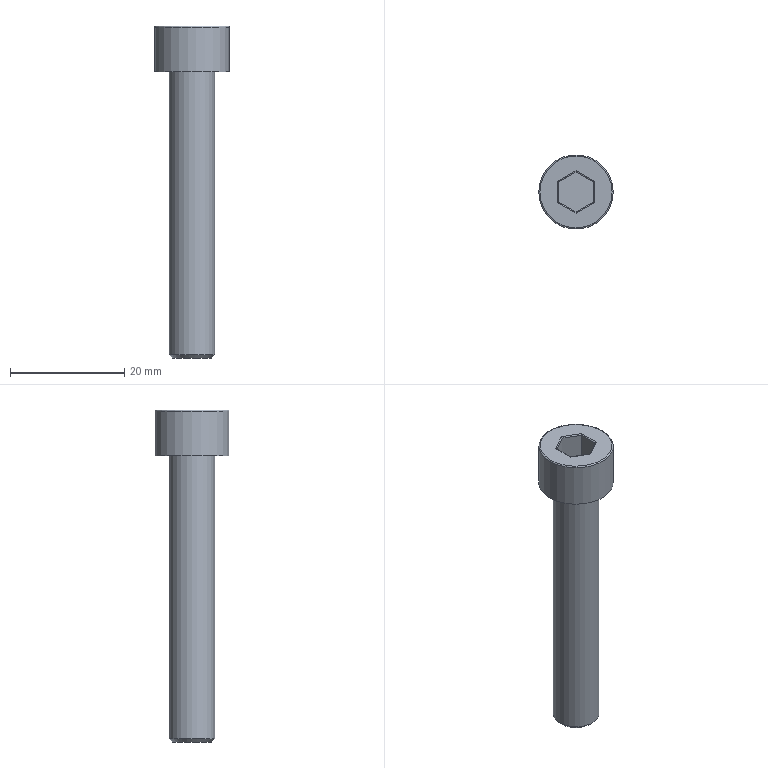Part | STEP file | 200 mesh_id666_x | 1 solid | 20 faces | box 13 x 13 x 58 mm | volume 3414 mm3 | plane 10 | cylinder 8 | torus 1 | cone 1 | commonest cylinder face diameters 0.4 x6 8 x1 13 x1
STEP:
#1=CARTESIAN_POINT('',(-16684.084,-4164.367,41.2));
#2=VERTEX_POINT('',#1);
#3=CARTESIAN_POINT('',(-16680.884,-4166.214,41.2));
#4=VERTEX_POINT('',#3);
#5=CARTESIAN_POINT('',(-16680.984,-4166.156,41.2));
#6=DIRECTION('',(0.866,-0.5,0.));
#7=VECTOR('',#6,1.);
#8=LINE('',#5,#7);
#9=EDGE_CURVE('',#2,#4,#8,.T.);
#10=ORIENTED_EDGE('',*,*,#9,.F.);
#11=CARTESIAN_POINT('',(-16684.084,-4160.672,41.2));
#12=VERTEX_POINT('',#11);
#13=CARTESIAN_POINT('',(-16684.084,-4164.251,41.2));
#14=DIRECTION('',(0.,-1.,0.));
#15=VECTOR('',#14,1.);
#16=LINE('',#13,#15);
#17=EDGE_CURVE('',#12,#2,#16,.T.);
#18=ORIENTED_EDGE('',*,*,#17,.F.);
#19=CARTESIAN_POINT('',(-16680.884,-4158.824,41.2));
#20=VERTEX_POINT('',#19);
#21=CARTESIAN_POINT('',(-16683.984,-4160.614,41.2));
#22=DIRECTION('',(-0.866,-0.5,0.));
#23=VECTOR('',#22,1.);
#24=LINE('',#21,#23);
#25=EDGE_CURVE('',#20,#12,#24,.T.);
#26=ORIENTED_EDGE('',*,*,#25,.F.);
#27=CARTESIAN_POINT('',(-16677.684,-4160.672,41.2));
#28=VERTEX_POINT('',#27);
#29=CARTESIAN_POINT('',(-16680.784,-4158.882,41.2));
#30=DIRECTION('',(-0.866,0.5,0.));
#31=VECTOR('',#30,1.);
#32=LINE('',#29,#31);
#33=EDGE_CURVE('',#28,#20,#32,.T.);
#34=ORIENTED_EDGE('',*,*,#33,.F.);
#35=CARTESIAN_POINT('',(-16677.684,-4164.367,41.2));
#36=VERTEX_POINT('',#35);
#37=CARTESIAN_POINT('',(-16677.684,-4160.787,41.2));
#38=DIRECTION('',(0.,1.,0.));
#39=VECTOR('',#38,1.);
#40=LINE('',#37,#39);
#41=EDGE_CURVE('',#36,#28,#40,.T.);
#42=ORIENTED_EDGE('',*,*,#41,.F.);
#43=CARTESIAN_POINT('',(-16677.784,-4164.424,41.2));
#44=DIRECTION('',(0.866,0.5,0.));
#45=VECTOR('',#44,1.);
#46=LINE('',#43,#45);
#47=EDGE_CURVE('',#4,#36,#46,.T.);
#48=ORIENTED_EDGE('',*,*,#47,.F.);
#49=EDGE_LOOP('',(#10,#18,#26,#34,#42,#48));
#50=FACE_BOUND('',#49,.T.);
#51=CARTESIAN_POINT('',(-16674.584,-4162.519,41.2));
#52=VERTEX_POINT('',#51);
#53=CARTESIAN_POINT('',(-16680.884,-4162.519,41.2));
#54=DIRECTION('',(0.,0.,-1.));
#55=DIRECTION('',(1.,0.,0.));
#56=AXIS2_PLACEMENT_3D('',#53,#54,#55);
#57=CIRCLE('',#56,6.3);
#58=EDGE_CURVE('',#52,#52,#57,.T.);
#59=ORIENTED_EDGE('',*,*,#58,.F.);
#60=EDGE_LOOP('',(#59));
#61=FACE_BOUND('',#60,.T.);
#62=CARTESIAN_POINT('',(-16680.884,-4162.519,41.2));
#63=DIRECTION('',(0.,0.,1.));
#64=DIRECTION('',(1.,0.,0.));
#65=AXIS2_PLACEMENT_3D('',#62,#63,#64);
#66=PLANE('',#65);
#67=ADVANCED_FACE('',(#50,#61),#66,.T.);
#68=CARTESIAN_POINT('',(-16684.884,-4162.519,-16.2));
#69=VERTEX_POINT('',#68);
#70=CARTESIAN_POINT('',(-16680.884,-4162.519,-16.2));
#71=DIRECTION('',(0.,0.,1.));
#72=DIRECTION('',(-1.,0.,0.));
#73=AXIS2_PLACEMENT_3D('',#70,#71,#72);
#74=CIRCLE('',#73,4.);
#75=EDGE_CURVE('',#69,#69,#74,.T.);
#76=ORIENTED_EDGE('',*,*,#75,.T.);
#77=EDGE_LOOP('',(#76));
#78=FACE_BOUND('',#77,.T.);
#79=CARTESIAN_POINT('',(-16684.884,-4162.519,33.2));
#80=VERTEX_POINT('',#79);
#81=CARTESIAN_POINT('',(-16680.884,-4162.519,33.2));
#82=DIRECTION('',(0.,0.,-1.));
#83=DIRECTION('',(-1.,0.,0.));
#84=AXIS2_PLACEMENT_3D('',#81,#82,#83);
#85=CIRCLE('',#84,4.);
#86=EDGE_CURVE('',#80,#80,#85,.T.);
#87=ORIENTED_EDGE('',*,*,#86,.T.);
#88=EDGE_LOOP('',(#87));
#89=FACE_BOUND('',#88,.T.);
#90=CARTESIAN_POINT('',(-16680.884,-4162.519,33.2));
#91=DIRECTION('',(0.,0.,-1.));
#92=DIRECTION('',(1.,0.,0.));
#93=AXIS2_PLACEMENT_3D('',#90,#91,#92);
#94=CYLINDRICAL_SURFACE('',#93,4.);
#95=ADVANCED_FACE('',(#78,#89),#94,.T.);
#96=ORIENTED_EDGE('',*,*,#86,.F.);
#97=EDGE_LOOP('',(#96));
#98=FACE_BOUND('',#97,.T.);
#99=CARTESIAN_POINT('',(-16687.384,-4162.519,33.2));
#100=VERTEX_POINT('',#99);
#101=CARTESIAN_POINT('',(-16680.884,-4162.519,33.2));
#102=DIRECTION('',(0.,0.,-1.));
#103=DIRECTION('',(-1.,0.,0.));
#104=AXIS2_PLACEMENT_3D('',#101,#102,#103);
#105=CIRCLE('',#104,6.5);
#106=EDGE_CURVE('',#100,#100,#105,.T.);
#107=ORIENTED_EDGE('',*,*,#106,.T.);
#108=EDGE_LOOP('',(#107));
#109=FACE_BOUND('',#108,.T.);
#110=CARTESIAN_POINT('',(-16680.884,-4162.519,33.2));
#111=DIRECTION('',(0.,0.,-1.));
#112=DIRECTION('',(-1.,0.,0.));
#113=AXIS2_PLACEMENT_3D('',#110,#111,#112);
#114=PLANE('',#113);
#115=ADVANCED_FACE('',(#98,#109),#114,.T.);
#116=CARTESIAN_POINT('',(-16674.384,-4162.519,41.));
#117=VERTEX_POINT('',#116);
#118=CARTESIAN_POINT('',(-16680.884,-4162.519,41.));
#119=DIRECTION('',(0.,0.,1.));
#120=DIRECTION('',(1.,0.,0.));
#121=AXIS2_PLACEMENT_3D('',#118,#119,#120);
#122=CIRCLE('',#121,6.5);
#123=EDGE_CURVE('',#117,#117,#122,.T.);
#124=ORIENTED_EDGE('',*,*,#123,.F.);
#125=EDGE_LOOP('',(#124));
#126=FACE_BOUND('',#125,.T.);
#127=ORIENTED_EDGE('',*,*,#106,.F.);
#128=EDGE_LOOP('',(#127));
#129=FACE_BOUND('',#128,.T.);
#130=CARTESIAN_POINT('',(-16680.884,-4162.519,33.2));
#131=DIRECTION('',(0.,0.,1.));
#132=DIRECTION('',(1.,0.,0.));
#133=AXIS2_PLACEMENT_3D('',#130,#131,#132);
#134=CYLINDRICAL_SURFACE('',#133,6.5);
#135=ADVANCED_FACE('',(#126,#129),#134,.T.);
#136=ORIENTED_EDGE('',*,*,#58,.T.);
#137=EDGE_LOOP('',(#136));
#138=FACE_BOUND('',#137,.T.);
#139=ORIENTED_EDGE('',*,*,#123,.T.);
#140=EDGE_LOOP('',(#139));
#141=FACE_BOUND('',#140,.T.);
#142=CARTESIAN_POINT('',(-16680.884,-4162.519,41.));
#143=DIRECTION('',(0.,0.,1.));
#144=DIRECTION('',(1.,0.,0.));
#145=AXIS2_PLACEMENT_3D('',#142,#143,#144);
#146=TOROIDAL_SURFACE('',#145,6.3,0.2);
#147=ADVANCED_FACE('',(#138,#141),#146,.T.);
#148=CARTESIAN_POINT('',(-16677.884,-4160.787,36.2));
#149=VERTEX_POINT('',#148);
#150=CARTESIAN_POINT('',(-16677.884,-4160.787,41.));
#151=VERTEX_POINT('',#150);
#152=CARTESIAN_POINT('',(-16677.884,-4160.787,41.2));
#153=DIRECTION('',(0.,0.,1.));
#154=VECTOR('',#153,1.);
#155=LINE('',#152,#154);
#156=EDGE_CURVE('',#149,#151,#155,.T.);
#157=ORIENTED_EDGE('',*,*,#156,.F.);
#158=CARTESIAN_POINT('',(-16677.884,-4164.251,36.2));
#159=VERTEX_POINT('',#158);
#160=CARTESIAN_POINT('',(-16677.884,-4164.251,36.2));
#161=DIRECTION('',(0.,-1.,0.));
#162=VECTOR('',#161,1.);
#163=LINE('',#160,#162);
#164=EDGE_CURVE('',#149,#159,#163,.T.);
#165=ORIENTED_EDGE('',*,*,#164,.T.);
#166=CARTESIAN_POINT('',(-16677.884,-4164.251,41.));
#167=VERTEX_POINT('',#166);
#168=CARTESIAN_POINT('',(-16677.884,-4164.251,41.2));
#169=DIRECTION('',(0.,0.,1.));
#170=VECTOR('',#169,1.);
#171=LINE('',#168,#170);
#172=EDGE_CURVE('',#159,#167,#171,.T.);
#173=ORIENTED_EDGE('',*,*,#172,.T.);
#174=CARTESIAN_POINT('',(-16677.884,-4164.251,41.));
#175=DIRECTION('',(0.,-1.,0.));
#176=VECTOR('',#175,1.);
#177=LINE('',#174,#176);
#178=EDGE_CURVE('',#151,#167,#177,.T.);
#179=ORIENTED_EDGE('',*,*,#178,.F.);
#180=EDGE_LOOP('',(#157,#165,#173,#179));
#181=FACE_OUTER_BOUND('',#180,.T.);
#182=CARTESIAN_POINT('',(-16677.884,-4164.251,41.2));
#183=DIRECTION('',(1.,0.,0.));
#184=DIRECTION('',(0.,0.,-1.));
#185=AXIS2_PLACEMENT_3D('',#182,#183,#184);
#186=PLANE('',#185);
#187=ADVANCED_FACE('',(#181),#186,.F.);
#188=CARTESIAN_POINT('',(-16680.884,-4159.055,36.2));
#189=VERTEX_POINT('',#188);
#190=CARTESIAN_POINT('',(-16680.884,-4159.055,41.));
#191=VERTEX_POINT('',#190);
#192=CARTESIAN_POINT('',(-16680.884,-4159.055,41.2));
#193=DIRECTION('',(0.,0.,1.));
#194=VECTOR('',#193,1.);
#195=LINE('',#192,#194);
#196=EDGE_CURVE('',#189,#191,#195,.T.);
#197=ORIENTED_EDGE('',*,*,#196,.F.);
#198=CARTESIAN_POINT('',(-16677.884,-4160.787,36.2));
#199=DIRECTION('',(0.866,-0.5,0.));
#200=VECTOR('',#199,1.);
#201=LINE('',#198,#200);
#202=EDGE_CURVE('',#189,#149,#201,.T.);
#203=ORIENTED_EDGE('',*,*,#202,.T.);
#204=ORIENTED_EDGE('',*,*,#156,.T.);
#205=CARTESIAN_POINT('',(-16677.884,-4160.787,41.));
#206=DIRECTION('',(0.866,-0.5,0.));
#207=VECTOR('',#206,1.);
#208=LINE('',#205,#207);
#209=EDGE_CURVE('',#191,#151,#208,.T.);
#210=ORIENTED_EDGE('',*,*,#209,.F.);
#211=EDGE_LOOP('',(#197,#203,#204,#210));
#212=FACE_OUTER_BOUND('',#211,.T.);
#213=CARTESIAN_POINT('',(-16677.884,-4160.787,41.2));
#214=DIRECTION('',(0.5,0.866,0.));
#215=DIRECTION('',(0.866,-0.5,0.));
#216=AXIS2_PLACEMENT_3D('',#213,#214,#215);
#217=PLANE('',#216);
#218=ADVANCED_FACE('',(#212),#217,.F.);
#219=CARTESIAN_POINT('',(-16683.884,-4160.787,36.2));
#220=VERTEX_POINT('',#219);
#221=CARTESIAN_POINT('',(-16683.884,-4160.787,41.));
#222=VERTEX_POINT('',#221);
#223=CARTESIAN_POINT('',(-16683.884,-4160.787,41.2));
#224=DIRECTION('',(0.,0.,1.));
#225=VECTOR('',#224,1.);
#226=LINE('',#223,#225);
#227=EDGE_CURVE('',#220,#222,#226,.T.);
#228=ORIENTED_EDGE('',*,*,#227,.F.);
#229=CARTESIAN_POINT('',(-16680.884,-4159.055,36.2));
#230=DIRECTION('',(0.866,0.5,0.));
#231=VECTOR('',#230,1.);
#232=LINE('',#229,#231);
#233=EDGE_CURVE('',#220,#189,#232,.T.);
#234=ORIENTED_EDGE('',*,*,#233,.T.);
#235=ORIENTED_EDGE('',*,*,#196,.T.);
#236=CARTESIAN_POINT('',(-16680.884,-4159.055,41.));
#237=DIRECTION('',(0.866,0.5,0.));
#238=VECTOR('',#237,1.);
#239=LINE('',#236,#238);
#240=EDGE_CURVE('',#222,#191,#239,.T.);
#241=ORIENTED_EDGE('',*,*,#240,.F.);
#242=EDGE_LOOP('',(#228,#234,#235,#241));
#243=FACE_OUTER_BOUND('',#242,.T.);
#244=CARTESIAN_POINT('',(-16680.884,-4159.055,41.2));
#245=DIRECTION('',(-0.5,0.866,0.));
#246=DIRECTION('',(0.866,0.5,0.));
#247=AXIS2_PLACEMENT_3D('',#244,#245,#246);
#248=PLANE('',#247);
#249=ADVANCED_FACE('',(#243),#248,.F.);
#250=CARTESIAN_POINT('',(-16683.884,-4164.251,36.2));
#251=VERTEX_POINT('',#250);
#252=CARTESIAN_POINT('',(-16683.884,-4164.251,41.));
#253=VERTEX_POINT('',#252);
#254=CARTESIAN_POINT('',(-16683.884,-4164.251,41.2));
#255=DIRECTION('',(0.,0.,1.));
#256=VECTOR('',#255,1.);
#257=LINE('',#254,#256);
#258=EDGE_CURVE('',#251,#253,#257,.T.);
#259=ORIENTED_EDGE('',*,*,#258,.F.);
#260=CARTESIAN_POINT('',(-16683.884,-4160.787,36.2));
#261=DIRECTION('',(0.,1.,0.));
#262=VECTOR('',#261,1.);
#263=LINE('',#260,#262);
#264=EDGE_CURVE('',#251,#220,#263,.T.);
#265=ORIENTED_EDGE('',*,*,#264,.T.);
#266=ORIENTED_EDGE('',*,*,#227,.T.);
#267=CARTESIAN_POINT('',(-16683.884,-4160.787,41.));
#268=DIRECTION('',(0.,1.,0.));
#269=VECTOR('',#268,1.);
#270=LINE('',#267,#269);
#271=EDGE_CURVE('',#253,#222,#270,.T.);
#272=ORIENTED_EDGE('',*,*,#271,.F.);
#273=EDGE_LOOP('',(#259,#265,#266,#272));
#274=FACE_OUTER_BOUND('',#273,.T.);
#275=CARTESIAN_POINT('',(-16683.884,-4160.787,41.2));
#276=DIRECTION('',(-1.,0.,0.));
#277=DIRECTION('',(0.,0.,1.));
#278=AXIS2_PLACEMENT_3D('',#275,#276,#277);
#279=PLANE('',#278);
#280=ADVANCED_FACE('',(#274),#279,.F.);
#281=CARTESIAN_POINT('',(-16680.884,-4165.983,36.2));
#282=VERTEX_POINT('',#281);
#283=CARTESIAN_POINT('',(-16680.884,-4165.983,41.));
#284=VERTEX_POINT('',#283);
#285=CARTESIAN_POINT('',(-16680.884,-4165.983,41.2));
#286=DIRECTION('',(0.,0.,1.));
#287=VECTOR('',#286,1.);
#288=LINE('',#285,#287);
#289=EDGE_CURVE('',#282,#284,#288,.T.);
#290=ORIENTED_EDGE('',*,*,#289,.F.);
#291=CARTESIAN_POINT('',(-16683.884,-4164.251,36.2));
#292=DIRECTION('',(-0.866,0.5,0.));
#293=VECTOR('',#292,1.);
#294=LINE('',#291,#293);
#295=EDGE_CURVE('',#282,#251,#294,.T.);
#296=ORIENTED_EDGE('',*,*,#295,.T.);
#297=ORIENTED_EDGE('',*,*,#258,.T.);
#298=CARTESIAN_POINT('',(-16683.884,-4164.251,41.));
#299=DIRECTION('',(-0.866,0.5,0.));
#300=VECTOR('',#299,1.);
#301=LINE('',#298,#300);
#302=EDGE_CURVE('',#284,#253,#301,.T.);
#303=ORIENTED_EDGE('',*,*,#302,.F.);
#304=EDGE_LOOP('',(#290,#296,#297,#303));
#305=FACE_OUTER_BOUND('',#304,.T.);
#306=CARTESIAN_POINT('',(-16683.884,-4164.251,41.2));
#307=DIRECTION('',(-0.5,-0.866,0.));
#308=DIRECTION('',(-0.866,0.5,0.));
#309=AXIS2_PLACEMENT_3D('',#306,#307,#308);
#310=PLANE('',#309);
#311=ADVANCED_FACE('',(#305),#310,.F.);
#312=ORIENTED_EDGE('',*,*,#172,.F.);
#313=CARTESIAN_POINT('',(-16680.884,-4165.983,36.2));
#314=DIRECTION('',(-0.866,-0.5,0.));
#315=VECTOR('',#314,1.);
#316=LINE('',#313,#315);
#317=EDGE_CURVE('',#159,#282,#316,.T.);
#318=ORIENTED_EDGE('',*,*,#317,.T.);
#319=ORIENTED_EDGE('',*,*,#289,.T.);
#320=CARTESIAN_POINT('',(-16680.884,-4165.983,41.));
#321=DIRECTION('',(-0.866,-0.5,0.));
#322=VECTOR('',#321,1.);
#323=LINE('',#320,#322);
#324=EDGE_CURVE('',#167,#284,#323,.T.);
#325=ORIENTED_EDGE('',*,*,#324,.F.);
#326=EDGE_LOOP('',(#312,#318,#319,#325));
#327=FACE_OUTER_BOUND('',#326,.T.);
#328=CARTESIAN_POINT('',(-16680.884,-4165.983,41.2));
#329=DIRECTION('',(0.5,-0.866,0.));
#330=DIRECTION('',(-0.866,-0.5,0.));
#331=AXIS2_PLACEMENT_3D('',#328,#329,#330);
#332=PLANE('',#331);
#333=ADVANCED_FACE('',(#327),#332,.F.);
#334=ORIENTED_EDGE('',*,*,#164,.F.);
#335=ORIENTED_EDGE('',*,*,#202,.F.);
#336=ORIENTED_EDGE('',*,*,#233,.F.);
#337=ORIENTED_EDGE('',*,*,#264,.F.);
#338=ORIENTED_EDGE('',*,*,#295,.F.);
#339=ORIENTED_EDGE('',*,*,#317,.F.);
#340=EDGE_LOOP('',(#334,#335,#336,#337,#338,#339));
#341=FACE_OUTER_BOUND('',#340,.T.);
#342=CARTESIAN_POINT('',(-51.5,-8040.538,36.2));
#343=DIRECTION('',(0.,0.,-1.));
#344=DIRECTION('',(-1.,0.,0.));
#345=AXIS2_PLACEMENT_3D('',#342,#343,#344);
#346=PLANE('',#345);
#347=ADVANCED_FACE('',(#341),#346,.F.);
#348=CARTESIAN_POINT('',(-16680.884,-4158.824,41.));
#349=DIRECTION('',(-1.,0.,0.));
#350=DIRECTION('',(0.,-1.,0.));
#351=AXIS2_PLACEMENT_3D('',#348,#349,#350);
#352=ELLIPSE('',#351,0.2309,0.2);
#353=EDGE_CURVE('',#191,#20,#352,.T.);
#354=ORIENTED_EDGE('',*,*,#353,.T.);
#355=ORIENTED_EDGE('',*,*,#25,.T.);
#356=CARTESIAN_POINT('',(-16684.084,-4160.672,41.));
#357=DIRECTION('',(0.5,0.866,0.));
#358=DIRECTION('',(0.866,-0.5,0.));
#359=AXIS2_PLACEMENT_3D('',#356,#357,#358);
#360=ELLIPSE('',#359,0.2309,0.2);
#361=EDGE_CURVE('',#12,#222,#360,.T.);
#362=ORIENTED_EDGE('',*,*,#361,.T.);
#363=ORIENTED_EDGE('',*,*,#240,.T.);
#364=EDGE_LOOP('',(#354,#355,#362,#363));
#365=FACE_OUTER_BOUND('',#364,.T.);
#366=CARTESIAN_POINT('',(-16682.484,-4159.748,41.));
#367=DIRECTION('',(0.866,0.5,0.));
#368=DIRECTION('',(0.5,-0.866,0.));
#369=AXIS2_PLACEMENT_3D('',#366,#367,#368);
#370=CYLINDRICAL_SURFACE('',#369,0.2);
#371=ADVANCED_FACE('',(#365),#370,.T.);
#372=ORIENTED_EDGE('',*,*,#361,.F.);
#373=ORIENTED_EDGE('',*,*,#17,.T.);
#374=CARTESIAN_POINT('',(-16684.084,-4164.367,41.));
#375=DIRECTION('',(-0.5,0.866,0.));
#376=DIRECTION('',(0.866,0.5,0.));
#377=AXIS2_PLACEMENT_3D('',#374,#375,#376);
#378=ELLIPSE('',#377,0.2309,0.2);
#379=EDGE_CURVE('',#2,#253,#378,.T.);
#380=ORIENTED_EDGE('',*,*,#379,.T.);
#381=ORIENTED_EDGE('',*,*,#271,.T.);
#382=EDGE_LOOP('',(#372,#373,#380,#381));
#383=FACE_OUTER_BOUND('',#382,.T.);
#384=CARTESIAN_POINT('',(-16684.084,-4162.519,41.));
#385=DIRECTION('',(0.,1.,0.));
#386=DIRECTION('',(0.,0.,-1.));
#387=AXIS2_PLACEMENT_3D('',#384,#385,#386);
#388=CYLINDRICAL_SURFACE('',#387,0.2);
#389=ADVANCED_FACE('',(#383),#388,.T.);
#390=ORIENTED_EDGE('',*,*,#353,.F.);
#391=ORIENTED_EDGE('',*,*,#209,.T.);
#392=CARTESIAN_POINT('',(-16677.684,-4160.672,41.));
#393=DIRECTION('',(-0.5,0.866,0.));
#394=DIRECTION('',(-0.866,-0.5,0.));
#395=AXIS2_PLACEMENT_3D('',#392,#393,#394);
#396=ELLIPSE('',#395,0.2309,0.2);
#397=EDGE_CURVE('',#151,#28,#396,.T.);
#398=ORIENTED_EDGE('',*,*,#397,.T.);
#399=ORIENTED_EDGE('',*,*,#33,.T.);
#400=EDGE_LOOP('',(#390,#391,#398,#399));
#401=FACE_OUTER_BOUND('',#400,.T.);
#402=CARTESIAN_POINT('',(-16679.284,-4159.748,41.));
#403=DIRECTION('',(0.866,-0.5,0.));
#404=DIRECTION('',(-0.5,-0.866,0.));
#405=AXIS2_PLACEMENT_3D('',#402,#403,#404);
#406=CYLINDRICAL_SURFACE('',#405,0.2);
#407=ADVANCED_FACE('',(#401),#406,.T.);
#408=ORIENTED_EDGE('',*,*,#379,.F.);
#409=ORIENTED_EDGE('',*,*,#9,.T.);
#410=CARTESIAN_POINT('',(-16680.884,-4166.214,41.));
#411=DIRECTION('',(-1.,0.,0.));
#412=DIRECTION('',(0.,-1.,0.));
#413=AXIS2_PLACEMENT_3D('',#410,#411,#412);
#414=ELLIPSE('',#413,0.2309,0.2);
#415=EDGE_CURVE('',#4,#284,#414,.T.);
#416=ORIENTED_EDGE('',*,*,#415,.T.);
#417=ORIENTED_EDGE('',*,*,#302,.T.);
#418=EDGE_LOOP('',(#408,#409,#416,#417));
#419=FACE_OUTER_BOUND('',#418,.T.);
#420=CARTESIAN_POINT('',(-16682.484,-4165.29,41.));
#421=DIRECTION('',(-0.866,0.5,0.));
#422=DIRECTION('',(0.5,0.866,0.));
#423=AXIS2_PLACEMENT_3D('',#420,#421,#422);
#424=CYLINDRICAL_SURFACE('',#423,0.2);
#425=ADVANCED_FACE('',(#419),#424,.T.);
#426=ORIENTED_EDGE('',*,*,#397,.F.);
#427=ORIENTED_EDGE('',*,*,#178,.T.);
#428=CARTESIAN_POINT('',(-16677.684,-4164.367,41.));
#429=DIRECTION('',(0.5,0.866,0.));
#430=DIRECTION('',(-0.866,0.5,0.));
#431=AXIS2_PLACEMENT_3D('',#428,#429,#430);
#432=ELLIPSE('',#431,0.2309,0.2);
#433=EDGE_CURVE('',#167,#36,#432,.T.);
#434=ORIENTED_EDGE('',*,*,#433,.T.);
#435=ORIENTED_EDGE('',*,*,#41,.T.);
#436=EDGE_LOOP('',(#426,#427,#434,#435));
#437=FACE_OUTER_BOUND('',#436,.T.);
#438=CARTESIAN_POINT('',(-16677.684,-4162.519,41.));
#439=DIRECTION('',(0.,-1.,0.));
#440=DIRECTION('',(0.,0.,1.));
#441=AXIS2_PLACEMENT_3D('',#438,#439,#440);
#442=CYLINDRICAL_SURFACE('',#441,0.2);
#443=ADVANCED_FACE('',(#437),#442,.T.);
#444=ORIENTED_EDGE('',*,*,#415,.F.);
#445=ORIENTED_EDGE('',*,*,#47,.T.);
#446=ORIENTED_EDGE('',*,*,#433,.F.);
#447=ORIENTED_EDGE('',*,*,#324,.T.);
#448=EDGE_LOOP('',(#444,#445,#446,#447));
#449=FACE_OUTER_BOUND('',#448,.T.);
#450=CARTESIAN_POINT('',(-16679.284,-4165.29,41.));
#451=DIRECTION('',(-0.866,-0.5,0.));
#452=DIRECTION('',(-0.5,0.866,0.));
#453=AXIS2_PLACEMENT_3D('',#450,#451,#452);
#454=CYLINDRICAL_SURFACE('',#453,0.2);
#455=ADVANCED_FACE('',(#449),#454,.T.);
#456=CARTESIAN_POINT('',(-16684.284,-4162.519,-16.8));
#457=VERTEX_POINT('',#456);
#458=CARTESIAN_POINT('',(-16680.884,-4162.519,-16.8));
#459=DIRECTION('',(0.,0.,-1.));
#460=DIRECTION('',(-1.,0.,0.));
#461=AXIS2_PLACEMENT_3D('',#458,#459,#460);
#462=CIRCLE('',#461,3.4);
#463=EDGE_CURVE('',#457,#457,#462,.T.);
#464=ORIENTED_EDGE('',*,*,#463,.T.);
#465=EDGE_LOOP('',(#464));
#466=FACE_OUTER_BOUND('',#465,.T.);
#467=CARTESIAN_POINT('',(-16680.884,-4162.519,-16.8));
#468=DIRECTION('',(0.,0.,-1.));
#469=DIRECTION('',(-1.,0.,0.));
#470=AXIS2_PLACEMENT_3D('',#467,#468,#469);
#471=PLANE('',#470);
#472=ADVANCED_FACE('',(#466),#471,.T.);
#473=ORIENTED_EDGE('',*,*,#463,.F.);
#474=EDGE_LOOP('',(#473));
#475=FACE_BOUND('',#474,.T.);
#476=ORIENTED_EDGE('',*,*,#75,.F.);
#477=EDGE_LOOP('',(#476));
#478=FACE_BOUND('',#477,.T.);
#479=CARTESIAN_POINT('',(-16680.884,-4162.519,-16.2));
#480=DIRECTION('',(0.,0.,1.));
#481=DIRECTION('',(1.,0.,0.));
#482=AXIS2_PLACEMENT_3D('',#479,#480,#481);
#483=CONICAL_SURFACE('',#482,4.,45.);
#484=ADVANCED_FACE('',(#475,#478),#483,.T.);
#485=CLOSED_SHELL('',(#67,#95,#115,#135,#147,#187,#218,#249,#280,#311,#333,#347,#371,#389,#407,#425,#443,#455,#472,#484));
#486=MANIFOLD_SOLID_BREP('',#485);
#487=(LENGTH_UNIT()NAMED_UNIT(*)SI_UNIT(.MILLI.,.METRE.));
#488=UNCERTAINTY_MEASURE_WITH_UNIT(LENGTH_MEASURE(0.00002),#487,'','');
#489=(NAMED_UNIT(*)PLANE_ANGLE_UNIT()SI_UNIT($,.RADIAN.));
#490=PLANE_ANGLE_MEASURE_WITH_UNIT(PLANE_ANGLE_MEASURE(0.01745),#489);
#491=DIMENSIONAL_EXPONENTS(0.,0.,0.,0.,0.,0.,0.);
#492=(CONVERSION_BASED_UNIT('DEGREE',#490)NAMED_UNIT(#491)PLANE_ANGLE_UNIT());
#493=(NAMED_UNIT(*)SI_UNIT($,.STERADIAN.)SOLID_ANGLE_UNIT());
#494=(GEOMETRIC_REPRESENTATION_CONTEXT(3)GLOBAL_UNCERTAINTY_ASSIGNED_CONTEXT((#488))GLOBAL_UNIT_ASSIGNED_CONTEXT((#487,#492,#493))REPRESENTATION_CONTEXT('',''));
#495=ADVANCED_BREP_SHAPE_REPRESENTATION('',(#486),#494);